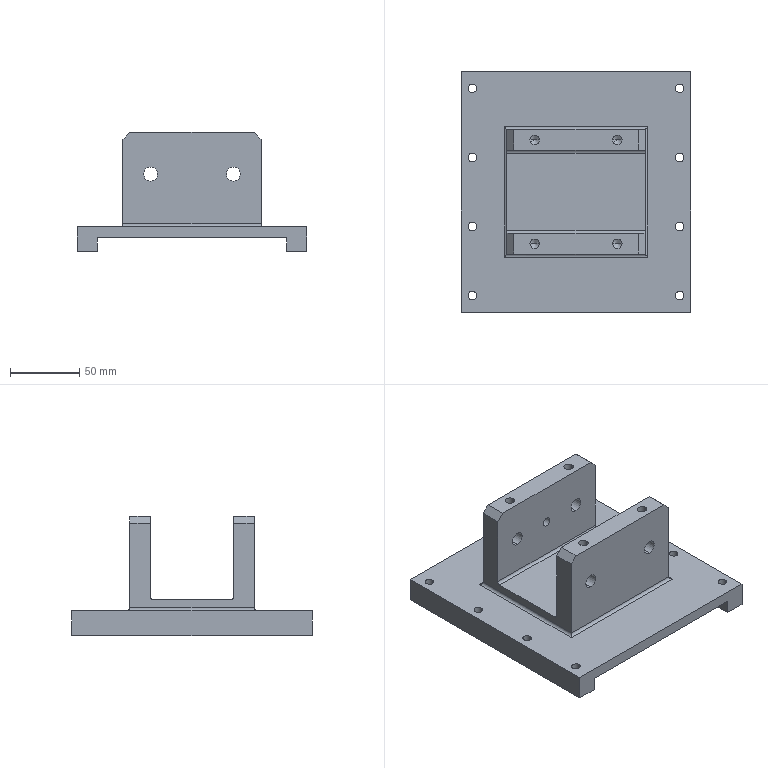NC program | NX | posted with a generic post | part box 166 x 174 x 86.2 mm
Lines 4421 to 4531 of 4531:
(DRILLING , TOOL : 倒角D10-90度)
N8750 T03 M6
N8752 G53
N8754 G17 G0 G90 X-37.6 Y30. B0. C0. S1200 M3
N8756 G43 Z30. H3
N8758 G94 G81 G98 Z-1.5 F100. R3.
N8760 Y-30.
N8762 X37.6
N8764 Y30.
N8766 G80
N8768 G0 X37.6 Y30. Z30.
N8770 M5
(DRILLING_COPY , TOOL : 钻头D6.8-73-105)
N8772 T04 M6
N8774 G53
N8776 G17 G0 G90 X-37.6 Y30. B0. C0. S1200 M3
N8778 G43 Z30. H4
N8780 G94 G83 G98 Z-22. F100. Q3. R3.
N8782 Y-30.
N8784 X37.6
N8786 Y30.
N8788 G80
N8790 G0 X37.6 Y30. Z30.
N8792 M5
(DRILLING_COPY_1 , TOOL : 倒角D10-90度)
N8794 T03 M6
N8796 G53
N8798 G17 G0 G90 X-37.6 Y30. B0. C0. S1200 M3
N8800 G43 Z30. H3
N8802 G94 G81 G98 Z-4.1 F100. R3.
N8804 Y-30.
N8806 X37.6
N8808 Y30.
N8810 G80
N8812 G0 X37.6 Y30. Z30.
(PLANAR_MILL_3 , TOOL : 倒角D10-90度)
N8814 X-46.9 Y-52. S3000
N8816 Z1.
N8818 G1 Z-2. F1000.
N8820 Y-45.
N8822 Y45.
N8824 Y52.
N8826 Z1.
N8828 G0 Z30.
N8830 X-28.3
N8832 Z1.
N8834 G1 Z-2.
N8836 Y45.
N8838 Y-45.
N8840 Y-52.
N8842 Z1.
N8844 G0 Z30.
N8846 X28.3
N8848 Z1.
N8850 G1 Z-2.
N8852 Y-45.
N8854 Y45.
N8856 Y52.
N8858 Z1.
N8860 G0 Z30.
N8862 X46.9
N8864 Z1.
N8866 G1 Z-2.
N8868 Y45.
N8870 Y-45.
N8872 Y-52.
N8874 Z1.
N8876 G0 Z30.
(PLANAR_MILL_3_COPY , TOOL : 倒角D10-90度)
N8878 X0. Y89.8
N8880 Z-67.2
N8882 G1 Z-70.2
N8884 Y84.8
N8886 X86.8
N8888 G2 X88.8 Y82.8 R2.
N8890 G1 Y-82.8
N8892 G2 X86.8 Y-84.8 R2.
N8894 G1 X-86.8
N8896 G2 X-88.8 Y-82.8 R2.
N8898 G1 Y82.8
N8900 G2 X-86.8 Y84.8 R2.
N8902 G1 X0.
N8904 Y89.8
N8906 Z-67.2
N8908 G0 Z30.
N8910 M5
(DRILLING_COPY_COPY , TOOL : 上排M8-28-D6.2-70)
N8912 T05 M6
N8914 G53
N8916 G17 G0 G90 X-37.6 Y30. B0. C0. S300 M3
N8918 G43 Z30. H5
N8920 G84 G94 G98 Z-5. F375. R3.
N8922 Y-30.
N8924 X37.6
N8926 Y30.
N8928 G80
N8930 G0 X37.6 Y30. Z30.
N8932 M5
N8934 M2